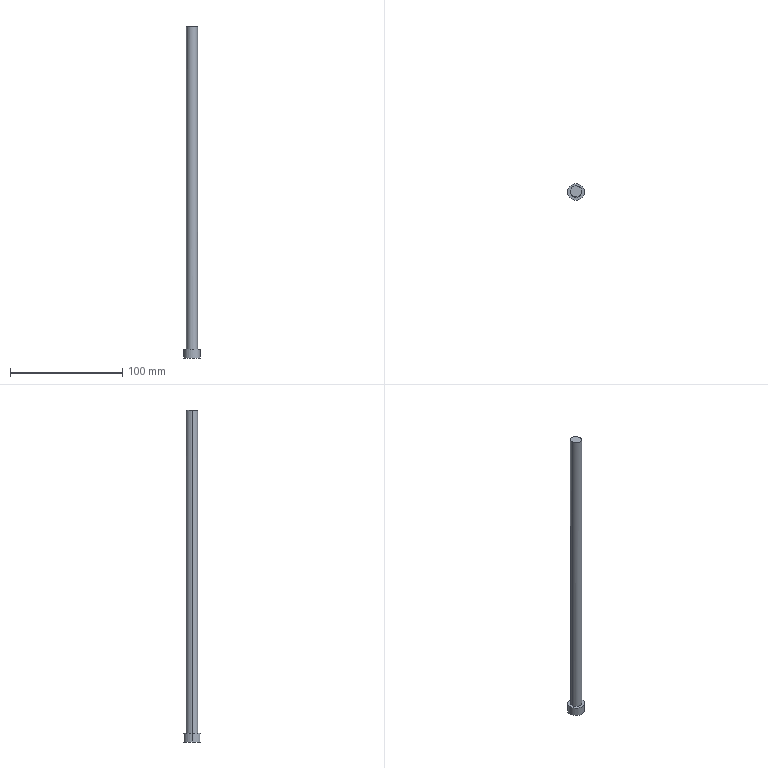Part | Creo | 1 solid | 10 faces | box 15 x 15 x 295.401 mm | volume 23917 mm3 | cylinder 6 | plane 4 | commonest cylinder face diameters 3 x2 10 x2 15 x2
STEP:
#1=CARTESIAN_POINT('',(31.,-137.,-252.5));
#2=VERTEX_POINT('',#1);
#3=CARTESIAN_POINT('',(21.,-137.,-252.5));
#4=VERTEX_POINT('',#3);
#5=CARTESIAN_POINT('',(26.,-137.,-252.5));
#6=DIRECTION('',(0.,0.,-1.));
#7=DIRECTION('',(1.,0.,0.));
#8=AXIS2_PLACEMENT_3D('',#5,#6,#7);
#9=CIRCLE('',#8,5.);
#10=EDGE_CURVE('',#2,#4,#9,.T.);
#11=ORIENTED_EDGE('',*,*,#10,.T.);
#12=CARTESIAN_POINT('',(21.,-137.,34.901));
#13=VERTEX_POINT('',#12);
#14=CARTESIAN_POINT('',(21.,-137.,34.901));
#15=DIRECTION('',(0.,0.,-1.));
#16=VECTOR('',#15,287.401);
#17=LINE('',#14,#16);
#18=EDGE_CURVE('',#13,#4,#17,.T.);
#19=ORIENTED_EDGE('',*,*,#18,.F.);
#20=CARTESIAN_POINT('',(31.,-137.,34.519));
#21=VERTEX_POINT('',#20);
#22=CARTESIAN_POINT('',(21.,-137.,34.901));
#23=CARTESIAN_POINT('',(21.,-137.589,34.901));
#24=CARTESIAN_POINT('',(21.215,-138.862,34.893));
#25=CARTESIAN_POINT('',(22.355,-140.641,34.849));
#26=CARTESIAN_POINT('',(24.15,-141.786,34.781));
#27=CARTESIAN_POINT('',(26.,-142.107,34.71));
#28=CARTESIAN_POINT('',(27.85,-141.786,34.64));
#29=CARTESIAN_POINT('',(29.645,-140.641,34.571));
#30=CARTESIAN_POINT('',(30.785,-138.862,34.528));
#31=CARTESIAN_POINT('',(31.,-137.589,34.519));
#32=CARTESIAN_POINT('',(31.,-137.,34.519));
#33=B_SPLINE_CURVE_WITH_KNOTS('',3,(#22,#23,#24,#25,#26,#27,#28,#29,#30,#31,#32),.UNSPECIFIED.,.F.,.F.,(4,1,1,1,1,1,1,1,4),(0.,0.125,0.25,0.375,0.5,0.625,0.75,0.875,1.),.UNSPECIFIED.);
#34=EDGE_CURVE('',#13,#21,#33,.T.);
#35=ORIENTED_EDGE('',*,*,#34,.T.);
#36=CARTESIAN_POINT('',(31.,-137.,34.519));
#37=DIRECTION('',(0.,0.,-1.));
#38=VECTOR('',#37,287.019);
#39=LINE('',#36,#38);
#40=EDGE_CURVE('',#21,#2,#39,.T.);
#41=ORIENTED_EDGE('',*,*,#40,.T.);
#42=EDGE_LOOP('',(#11,#19,#35,#41));
#43=FACE_OUTER_BOUND('',#42,.F.);
#44=CARTESIAN_POINT('',(26.,-137.,135.));
#45=DIRECTION('',(0.,0.,-1.));
#46=DIRECTION('',(1.,0.,0.));
#47=AXIS2_PLACEMENT_3D('',#44,#45,#46);
#48=CYLINDRICAL_SURFACE('',#47,5.);
#49=ADVANCED_FACE('',(#43),#48,.T.);
#50=CARTESIAN_POINT('',(18.5,-137.,-252.5));
#51=VERTEX_POINT('',#50);
#52=CARTESIAN_POINT('',(33.5,-137.,-252.5));
#53=VERTEX_POINT('',#52);
#54=CARTESIAN_POINT('',(26.,-137.,-252.5));
#55=DIRECTION('',(0.,0.,1.));
#56=DIRECTION('',(-1.,0.,0.));
#57=AXIS2_PLACEMENT_3D('',#54,#55,#56);
#58=CIRCLE('',#57,7.5);
#59=EDGE_CURVE('',#51,#53,#58,.T.);
#60=ORIENTED_EDGE('',*,*,#59,.F.);
#61=CARTESIAN_POINT('',(26.,-137.,-252.5));
#62=DIRECTION('',(0.,0.,1.));
#63=DIRECTION('',(1.,0.,0.));
#64=AXIS2_PLACEMENT_3D('',#61,#62,#63);
#65=CIRCLE('',#64,7.5);
#66=EDGE_CURVE('',#53,#51,#65,.T.);
#67=ORIENTED_EDGE('',*,*,#66,.F.);
#68=EDGE_LOOP('',(#60,#67));
#69=FACE_OUTER_BOUND('',#68,.F.);
#70=CARTESIAN_POINT('',(26.,-137.,-252.5));
#71=DIRECTION('',(0.,0.,-1.));
#72=DIRECTION('',(-1.,0.,0.));
#73=AXIS2_PLACEMENT_3D('',#70,#71,#72);
#74=CIRCLE('',#73,5.);
#75=EDGE_CURVE('',#4,#2,#74,.T.);
#76=ORIENTED_EDGE('',*,*,#75,.F.);
#77=ORIENTED_EDGE('',*,*,#10,.F.);
#78=EDGE_LOOP('',(#76,#77));
#79=FACE_BOUND('',#78,.F.);
#80=CARTESIAN_POINT('',(26.,-137.,-252.5));
#81=DIRECTION('',(0.,0.,1.));
#82=DIRECTION('',(-1.,0.,0.));
#83=AXIS2_PLACEMENT_3D('',#80,#81,#82);
#84=PLANE('',#83);
#85=ADVANCED_FACE('',(#69,#79),#84,.T.);
#86=ORIENTED_EDGE('',*,*,#75,.T.);
#87=ORIENTED_EDGE('',*,*,#40,.F.);
#88=CARTESIAN_POINT('',(31.,-137.,34.519));
#89=CARTESIAN_POINT('',(31.,-136.411,34.519));
#90=CARTESIAN_POINT('',(30.785,-135.138,34.528));
#91=CARTESIAN_POINT('',(29.645,-133.359,34.571));
#92=CARTESIAN_POINT('',(27.85,-132.214,34.64));
#93=CARTESIAN_POINT('',(26.,-131.893,34.71));
#94=CARTESIAN_POINT('',(24.15,-132.214,34.781));
#95=CARTESIAN_POINT('',(22.355,-133.359,34.849));
#96=CARTESIAN_POINT('',(21.215,-135.138,34.893));
#97=CARTESIAN_POINT('',(21.,-136.411,34.901));
#98=CARTESIAN_POINT('',(21.,-137.,34.901));
#99=B_SPLINE_CURVE_WITH_KNOTS('',3,(#88,#89,#90,#91,#92,#93,#94,#95,#96,#97,#98),.UNSPECIFIED.,.F.,.F.,(4,1,1,1,1,1,1,1,4),(0.,0.125,0.25,0.375,0.5,0.625,0.75,0.875,1.),.UNSPECIFIED.);
#100=EDGE_CURVE('',#21,#13,#99,.T.);
#101=ORIENTED_EDGE('',*,*,#100,.T.);
#102=ORIENTED_EDGE('',*,*,#18,.T.);
#103=EDGE_LOOP('',(#86,#87,#101,#102));
#104=FACE_OUTER_BOUND('',#103,.F.);
#105=CARTESIAN_POINT('',(26.,-137.,135.));
#106=DIRECTION('',(0.,0.,-1.));
#107=DIRECTION('',(1.,0.,0.));
#108=AXIS2_PLACEMENT_3D('',#105,#106,#107);
#109=CYLINDRICAL_SURFACE('',#108,5.);
#110=ADVANCED_FACE('',(#104),#109,.T.);
#111=ORIENTED_EDGE('',*,*,#100,.F.);
#112=ORIENTED_EDGE('',*,*,#34,.F.);
#113=EDGE_LOOP('',(#111,#112));
#114=FACE_OUTER_BOUND('',#113,.F.);
#115=CARTESIAN_POINT('',(16.957,24.474,35.055));
#116=DIRECTION('',(0.03814,0.,0.9993));
#117=DIRECTION('',(0.9993,0.,-0.03814));
#118=AXIS2_PLACEMENT_3D('',#115,#116,#117);
#119=PLANE('',#118);
#120=ADVANCED_FACE('',(#114),#119,.T.);
#121=CARTESIAN_POINT('',(33.5,-137.,-258.));
#122=VERTEX_POINT('',#121);
#123=CARTESIAN_POINT('',(33.5,-137.,-255.));
#124=VERTEX_POINT('',#123);
#125=CARTESIAN_POINT('',(33.5,-137.,-258.));
#126=CARTESIAN_POINT('',(33.5,-137.205,-258.));
#127=CARTESIAN_POINT('',(33.484,-137.583,-257.922));
#128=CARTESIAN_POINT('',(33.425,-138.09,-257.589));
#129=CARTESIAN_POINT('',(33.365,-138.424,-257.085));
#130=CARTESIAN_POINT('',(33.34,-138.539,-256.497));
#131=CARTESIAN_POINT('',(33.365,-138.422,-255.912));
#132=CARTESIAN_POINT('',(33.425,-138.091,-255.413));
#133=CARTESIAN_POINT('',(33.484,-137.585,-255.078));
#134=CARTESIAN_POINT('',(33.5,-137.206,-255.));
#135=CARTESIAN_POINT('',(33.5,-137.,-255.));
#136=B_SPLINE_CURVE_WITH_KNOTS('',3,(#125,#126,#127,#128,#129,#130,#131,#132,#133,#134,#135),.UNSPECIFIED.,.F.,.F.,(4,1,1,1,1,1,1,1,4),(0.,0.125,0.25,0.375,0.5,0.625,0.75,0.875,1.),.UNSPECIFIED.);
#137=EDGE_CURVE('',#122,#124,#136,.T.);
#138=ORIENTED_EDGE('',*,*,#137,.F.);
#139=CARTESIAN_POINT('',(33.5,-137.,-260.5));
#140=VERTEX_POINT('',#139);
#141=CARTESIAN_POINT('',(33.5,-137.,-260.5));
#142=DIRECTION('',(0.,0.,1.));
#143=VECTOR('',#142,2.5);
#144=LINE('',#141,#143);
#145=EDGE_CURVE('',#140,#122,#144,.T.);
#146=ORIENTED_EDGE('',*,*,#145,.F.);
#147=CARTESIAN_POINT('',(18.5,-137.,-260.5));
#148=VERTEX_POINT('',#147);
#149=CARTESIAN_POINT('',(26.,-137.,-260.5));
#150=DIRECTION('',(0.,0.,-1.));
#151=DIRECTION('',(1.,0.,0.));
#152=AXIS2_PLACEMENT_3D('',#149,#150,#151);
#153=CIRCLE('',#152,7.5);
#154=EDGE_CURVE('',#140,#148,#153,.T.);
#155=ORIENTED_EDGE('',*,*,#154,.T.);
#156=CARTESIAN_POINT('',(18.5,-137.,-260.5));
#157=DIRECTION('',(0.,0.,1.));
#158=VECTOR('',#157,8.);
#159=LINE('',#156,#158);
#160=EDGE_CURVE('',#148,#51,#159,.T.);
#161=ORIENTED_EDGE('',*,*,#160,.T.);
#162=ORIENTED_EDGE('',*,*,#59,.T.);
#163=CARTESIAN_POINT('',(33.5,-137.,-255.));
#164=DIRECTION('',(0.000005138,0.,1.));
#165=VECTOR('',#164,2.5);
#166=LINE('',#163,#165);
#167=EDGE_CURVE('',#124,#53,#166,.T.);
#168=ORIENTED_EDGE('',*,*,#167,.F.);
#169=EDGE_LOOP('',(#138,#146,#155,#161,#162,#168));
#170=FACE_OUTER_BOUND('',#169,.F.);
#171=CARTESIAN_POINT('',(26.,-137.,-260.5));
#172=DIRECTION('',(0.,0.,1.));
#173=DIRECTION('',(-1.,0.,0.));
#174=AXIS2_PLACEMENT_3D('',#171,#172,#173);
#175=CYLINDRICAL_SURFACE('',#174,7.5);
#176=ADVANCED_FACE('',(#170),#175,.T.);
#177=ORIENTED_EDGE('',*,*,#137,.T.);
#178=CARTESIAN_POINT('',(26.,-137.,-255.));
#179=VERTEX_POINT('',#178);
#180=CARTESIAN_POINT('',(26.,-137.,-255.));
#181=DIRECTION('',(1.,0.,-0.000004561));
#182=VECTOR('',#181,7.5);
#183=LINE('',#180,#182);
#184=EDGE_CURVE('',#179,#124,#183,.T.);
#185=ORIENTED_EDGE('',*,*,#184,.F.);
#186=CARTESIAN_POINT('',(26.,-137.,-258.));
#187=VERTEX_POINT('',#186);
#188=CARTESIAN_POINT('',(26.,-137.,-256.5));
#189=DIRECTION('',(1.,0.,0.));
#190=DIRECTION('',(0.,0.,1.));
#191=AXIS2_PLACEMENT_3D('',#188,#189,#190);
#192=CIRCLE('',#191,1.5);
#193=EDGE_CURVE('',#179,#187,#192,.T.);
#194=ORIENTED_EDGE('',*,*,#193,.T.);
#195=CARTESIAN_POINT('',(26.,-137.,-258.));
#196=DIRECTION('',(1.,0.,0.));
#197=VECTOR('',#196,7.5);
#198=LINE('',#195,#197);
#199=EDGE_CURVE('',#187,#122,#198,.T.);
#200=ORIENTED_EDGE('',*,*,#199,.T.);
#201=EDGE_LOOP('',(#177,#185,#194,#200));
#202=FACE_OUTER_BOUND('',#201,.F.);
#203=CARTESIAN_POINT('',(26.,-137.,-256.5));
#204=DIRECTION('',(1.,0.,0.));
#205=DIRECTION('',(0.,0.,-1.));
#206=AXIS2_PLACEMENT_3D('',#203,#204,#205);
#207=CYLINDRICAL_SURFACE('',#206,1.5);
#208=ADVANCED_FACE('',(#202),#207,.F.);
#209=CARTESIAN_POINT('',(33.5,-137.,-255.));
#210=CARTESIAN_POINT('',(33.5,-136.794,-255.));
#211=CARTESIAN_POINT('',(33.484,-136.415,-255.078));
#212=CARTESIAN_POINT('',(33.424,-135.907,-255.414));
#213=CARTESIAN_POINT('',(33.364,-135.576,-255.917));
#214=CARTESIAN_POINT('',(33.34,-135.461,-256.506));
#215=CARTESIAN_POINT('',(33.365,-135.579,-257.089));
#216=CARTESIAN_POINT('',(33.424,-135.908,-257.586));
#217=CARTESIAN_POINT('',(33.484,-136.414,-257.922));
#218=CARTESIAN_POINT('',(33.5,-136.794,-258.));
#219=CARTESIAN_POINT('',(33.5,-137.,-258.));
#220=B_SPLINE_CURVE_WITH_KNOTS('',3,(#209,#210,#211,#212,#213,#214,#215,#216,#217,#218,#219),.UNSPECIFIED.,.F.,.F.,(4,1,1,1,1,1,1,1,4),(0.,0.125,0.25,0.375,0.5,0.625,0.75,0.875,1.),.UNSPECIFIED.);
#221=EDGE_CURVE('',#124,#122,#220,.T.);
#222=ORIENTED_EDGE('',*,*,#221,.T.);
#223=ORIENTED_EDGE('',*,*,#199,.F.);
#224=CARTESIAN_POINT('',(26.,-137.,-256.5));
#225=DIRECTION('',(1.,0.,0.));
#226=DIRECTION('',(0.,0.,-1.));
#227=AXIS2_PLACEMENT_3D('',#224,#225,#226);
#228=CIRCLE('',#227,1.5);
#229=EDGE_CURVE('',#187,#179,#228,.T.);
#230=ORIENTED_EDGE('',*,*,#229,.T.);
#231=ORIENTED_EDGE('',*,*,#184,.T.);
#232=EDGE_LOOP('',(#222,#223,#230,#231));
#233=FACE_OUTER_BOUND('',#232,.F.);
#234=CARTESIAN_POINT('',(26.,-137.,-256.5));
#235=DIRECTION('',(1.,0.,0.));
#236=DIRECTION('',(0.,0.,-1.));
#237=AXIS2_PLACEMENT_3D('',#234,#235,#236);
#238=CYLINDRICAL_SURFACE('',#237,1.5);
#239=ADVANCED_FACE('',(#233),#238,.F.);
#240=ORIENTED_EDGE('',*,*,#221,.F.);
#241=ORIENTED_EDGE('',*,*,#167,.T.);
#242=ORIENTED_EDGE('',*,*,#66,.T.);
#243=ORIENTED_EDGE('',*,*,#160,.F.);
#244=CARTESIAN_POINT('',(26.,-137.,-260.5));
#245=DIRECTION('',(0.,0.,-1.));
#246=DIRECTION('',(-1.,0.,0.));
#247=AXIS2_PLACEMENT_3D('',#244,#245,#246);
#248=CIRCLE('',#247,7.5);
#249=EDGE_CURVE('',#148,#140,#248,.T.);
#250=ORIENTED_EDGE('',*,*,#249,.T.);
#251=ORIENTED_EDGE('',*,*,#145,.T.);
#252=EDGE_LOOP('',(#240,#241,#242,#243,#250,#251));
#253=FACE_OUTER_BOUND('',#252,.F.);
#254=CARTESIAN_POINT('',(26.,-137.,-260.5));
#255=DIRECTION('',(0.,0.,1.));
#256=DIRECTION('',(-1.,0.,0.));
#257=AXIS2_PLACEMENT_3D('',#254,#255,#256);
#258=CYLINDRICAL_SURFACE('',#257,7.5);
#259=ADVANCED_FACE('',(#253),#258,.T.);
#260=ORIENTED_EDGE('',*,*,#154,.F.);
#261=ORIENTED_EDGE('',*,*,#249,.F.);
#262=EDGE_LOOP('',(#260,#261));
#263=FACE_OUTER_BOUND('',#262,.F.);
#264=CARTESIAN_POINT('',(288.714,5.015,-260.5));
#265=DIRECTION('',(0.,0.,-1.));
#266=DIRECTION('',(1.,0.,0.));
#267=AXIS2_PLACEMENT_3D('',#264,#265,#266);
#268=PLANE('',#267);
#269=ADVANCED_FACE('',(#263),#268,.T.);
#270=ORIENTED_EDGE('',*,*,#229,.F.);
#271=ORIENTED_EDGE('',*,*,#193,.F.);
#272=EDGE_LOOP('',(#270,#271));
#273=FACE_OUTER_BOUND('',#272,.F.);
#274=CARTESIAN_POINT('',(26.,-137.,-256.5));
#275=DIRECTION('',(-1.,0.,0.));
#276=DIRECTION('',(0.,0.,1.));
#277=AXIS2_PLACEMENT_3D('',#274,#275,#276);
#278=PLANE('',#277);
#279=ADVANCED_FACE('',(#273),#278,.F.);
#280=CLOSED_SHELL('',(#49,#85,#110,#120,#176,#208,#239,#259,#269,#279));
#281=MANIFOLD_SOLID_BREP('',#280);
#282=(LENGTH_UNIT()NAMED_UNIT(*)SI_UNIT(.MILLI.,.METRE.));
#283=UNCERTAINTY_MEASURE_WITH_UNIT(LENGTH_MEASURE(0.02961),#282,'','');
#284=(NAMED_UNIT(*)PLANE_ANGLE_UNIT()SI_UNIT($,.RADIAN.));
#285=PLANE_ANGLE_MEASURE_WITH_UNIT(PLANE_ANGLE_MEASURE(0.01745),#284);
#286=(CONVERSION_BASED_UNIT('DEGREE',#285)NAMED_UNIT(*)PLANE_ANGLE_UNIT());
#287=(NAMED_UNIT(*)SI_UNIT($,.STERADIAN.)SOLID_ANGLE_UNIT());
#288=(GEOMETRIC_REPRESENTATION_CONTEXT(3)GLOBAL_UNCERTAINTY_ASSIGNED_CONTEXT((#283))GLOBAL_UNIT_ASSIGNED_CONTEXT((#282,#286,#287))REPRESENTATION_CONTEXT('',''));
#289=ADVANCED_BREP_SHAPE_REPRESENTATION('',(#281),#288);